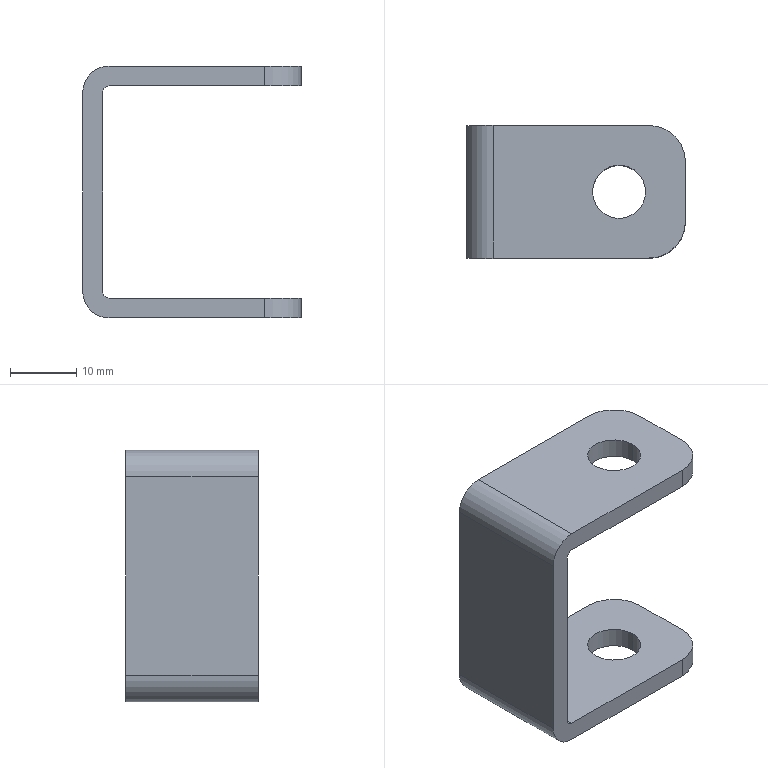Part | NX | features BLEND 1, DATUM_CSYS 1, EXTRACT_DATUM_PLANE 1, EXTRUDE 1, LINKED_BODY 1, SKETCH 1, SUBTRACT 1 | 1 solid | 22 faces | box 33 x 20 x 38 mm | volume 5372 mm3 | cylinder 12 | plane 10 | commonest cylinder face diameters 8 x6 11 x4 2 x2
STEP:
#1=CARTESIAN_POINT('',(-23.,10.,-15.));
#2=VERTEX_POINT('',#1);
#3=CARTESIAN_POINT('',(-23.,10.,15.));
#4=VERTEX_POINT('',#3);
#5=CARTESIAN_POINT('',(-23.,10.,-15.));
#6=DIRECTION('',(0.,0.,1.));
#7=VECTOR('',#6,1000.);
#8=LINE('',#5,#7);
#9=EDGE_CURVE('',#2,#4,#8,.T.);
#10=ORIENTED_EDGE('',*,*,#9,.F.);
#11=CARTESIAN_POINT('',(-23.,-10.,-15.));
#12=VERTEX_POINT('',#11);
#13=CARTESIAN_POINT('',(-23.,-10.,-15.));
#14=DIRECTION('',(0.,1.,0.));
#15=VECTOR('',#14,1000.);
#16=LINE('',#13,#15);
#17=EDGE_CURVE('',#12,#2,#16,.T.);
#18=ORIENTED_EDGE('',*,*,#17,.F.);
#19=CARTESIAN_POINT('',(-23.,-10.,15.));
#20=VERTEX_POINT('',#19);
#21=CARTESIAN_POINT('',(-23.,-10.,-15.));
#22=DIRECTION('',(0.,0.,1.));
#23=VECTOR('',#22,1000.);
#24=LINE('',#21,#23);
#25=EDGE_CURVE('',#12,#20,#24,.T.);
#26=ORIENTED_EDGE('',*,*,#25,.T.);
#27=CARTESIAN_POINT('',(-23.,-10.,15.));
#28=DIRECTION('',(0.,1.,0.));
#29=VECTOR('',#28,1000.);
#30=LINE('',#27,#29);
#31=EDGE_CURVE('',#20,#4,#30,.T.);
#32=ORIENTED_EDGE('',*,*,#31,.T.);
#33=EDGE_LOOP('',(#10,#18,#26,#32));
#34=FACE_BOUND('',#33,.T.);
#35=CARTESIAN_POINT('',(-23.,-10.,-15.));
#36=DIRECTION('',(-1.,0.,0.));
#37=DIRECTION('',(0.,0.,1.));
#38=AXIS2_PLACEMENT_3D('',#35,#36,#37);
#39=PLANE('',#38);
#40=ADVANCED_FACE('',(#34),#39,.T.);
#41=CARTESIAN_POINT('',(-19.,10.,19.));
#42=VERTEX_POINT('',#41);
#43=CARTESIAN_POINT('',(-19.,10.,15.));
#44=DIRECTION('',(0.,1.,0.));
#45=DIRECTION('',(-1.,0.,0.));
#46=AXIS2_PLACEMENT_3D('',#43,#44,#45);
#47=CIRCLE('',#46,4.);
#48=EDGE_CURVE('',#4,#42,#47,.T.);
#49=ORIENTED_EDGE('',*,*,#48,.F.);
#50=ORIENTED_EDGE('',*,*,#31,.F.);
#51=CARTESIAN_POINT('',(-19.,-10.,19.));
#52=VERTEX_POINT('',#51);
#53=CARTESIAN_POINT('',(-19.,-10.,15.));
#54=DIRECTION('',(0.,1.,0.));
#55=DIRECTION('',(-1.,0.,0.));
#56=AXIS2_PLACEMENT_3D('',#53,#54,#55);
#57=CIRCLE('',#56,4.);
#58=EDGE_CURVE('',#20,#52,#57,.T.);
#59=ORIENTED_EDGE('',*,*,#58,.T.);
#60=CARTESIAN_POINT('',(-19.,-10.,19.));
#61=DIRECTION('',(0.,1.,0.));
#62=VECTOR('',#61,1000.);
#63=LINE('',#60,#62);
#64=EDGE_CURVE('',#52,#42,#63,.T.);
#65=ORIENTED_EDGE('',*,*,#64,.T.);
#66=EDGE_LOOP('',(#49,#50,#59,#65));
#67=FACE_BOUND('',#66,.T.);
#68=CARTESIAN_POINT('',(-19.,-10.,15.));
#69=DIRECTION('',(0.,1.,0.));
#70=DIRECTION('',(0.,0.,1.));
#71=AXIS2_PLACEMENT_3D('',#68,#69,#70);
#72=CYLINDRICAL_SURFACE('',#71,4.);
#73=ADVANCED_FACE('',(#67),#72,.T.);
#74=CARTESIAN_POINT('',(4.5,-10.,19.));
#75=VERTEX_POINT('',#74);
#76=CARTESIAN_POINT('',(-19.,-10.,19.));
#77=DIRECTION('',(1.,0.,0.));
#78=VECTOR('',#77,1000.);
#79=LINE('',#76,#78);
#80=EDGE_CURVE('',#52,#75,#79,.T.);
#81=ORIENTED_EDGE('',*,*,#80,.T.);
#82=CARTESIAN_POINT('',(10.,-4.5,19.));
#83=VERTEX_POINT('',#82);
#84=CARTESIAN_POINT('',(4.5,-4.5,19.));
#85=DIRECTION('',(0.,0.,1.));
#86=DIRECTION('',(1.,0.,0.));
#87=AXIS2_PLACEMENT_3D('',#84,#85,#86);
#88=CIRCLE('',#87,5.5);
#89=EDGE_CURVE('',#75,#83,#88,.T.);
#90=ORIENTED_EDGE('',*,*,#89,.T.);
#91=CARTESIAN_POINT('',(10.,4.5,19.));
#92=VERTEX_POINT('',#91);
#93=CARTESIAN_POINT('',(10.,-10.,19.));
#94=DIRECTION('',(0.,1.,0.));
#95=VECTOR('',#94,1000.);
#96=LINE('',#93,#95);
#97=EDGE_CURVE('',#83,#92,#96,.T.);
#98=ORIENTED_EDGE('',*,*,#97,.T.);
#99=CARTESIAN_POINT('',(4.5,10.,19.));
#100=VERTEX_POINT('',#99);
#101=CARTESIAN_POINT('',(4.5,4.5,19.));
#102=DIRECTION('',(0.,0.,1.));
#103=DIRECTION('',(1.,0.,0.));
#104=AXIS2_PLACEMENT_3D('',#101,#102,#103);
#105=CIRCLE('',#104,5.5);
#106=EDGE_CURVE('',#92,#100,#105,.T.);
#107=ORIENTED_EDGE('',*,*,#106,.T.);
#108=CARTESIAN_POINT('',(5.,10.,19.));
#109=DIRECTION('',(1.,0.,0.));
#110=VECTOR('',#109,1000.);
#111=LINE('',#108,#110);
#112=EDGE_CURVE('',#42,#100,#111,.T.);
#113=ORIENTED_EDGE('',*,*,#112,.F.);
#114=ORIENTED_EDGE('',*,*,#64,.F.);
#115=EDGE_LOOP('',(#81,#90,#98,#107,#113,#114));
#116=FACE_BOUND('',#115,.T.);
#117=CARTESIAN_POINT('',(4.,0.,19.));
#118=VERTEX_POINT('',#117);
#119=CARTESIAN_POINT('',(-4.,0.,19.));
#120=VERTEX_POINT('',#119);
#121=CARTESIAN_POINT('',(0.,0.,19.));
#122=DIRECTION('',(0.,0.,1.));
#123=DIRECTION('',(1.,0.,0.));
#124=AXIS2_PLACEMENT_3D('',#121,#122,#123);
#125=CIRCLE('',#124,4.);
#126=EDGE_CURVE('',#118,#120,#125,.T.);
#127=ORIENTED_EDGE('',*,*,#126,.F.);
#128=CARTESIAN_POINT('',(0.,0.,19.));
#129=DIRECTION('',(0.,0.,1.));
#130=DIRECTION('',(-1.,0.,0.));
#131=AXIS2_PLACEMENT_3D('',#128,#129,#130);
#132=CIRCLE('',#131,4.);
#133=EDGE_CURVE('',#120,#118,#132,.T.);
#134=ORIENTED_EDGE('',*,*,#133,.F.);
#135=EDGE_LOOP('',(#127,#134));
#136=FACE_BOUND('',#135,.T.);
#137=CARTESIAN_POINT('',(5.,-10.,19.));
#138=DIRECTION('',(0.,0.,1.));
#139=DIRECTION('',(1.,0.,0.));
#140=AXIS2_PLACEMENT_3D('',#137,#138,#139);
#141=PLANE('',#140);
#142=ADVANCED_FACE('',(#116,#136),#141,.T.);
#143=ORIENTED_EDGE('',*,*,#97,.F.);
#144=CARTESIAN_POINT('',(10.,-4.5,16.));
#145=VERTEX_POINT('',#144);
#146=CARTESIAN_POINT('',(10.,-4.5,16.));
#147=DIRECTION('',(0.,0.,-1.));
#148=VECTOR('',#147,1000.);
#149=LINE('',#146,#148);
#150=EDGE_CURVE('',#83,#145,#149,.T.);
#151=ORIENTED_EDGE('',*,*,#150,.T.);
#152=CARTESIAN_POINT('',(10.,4.5,16.));
#153=VERTEX_POINT('',#152);
#154=CARTESIAN_POINT('',(10.,-10.,16.));
#155=DIRECTION('',(0.,1.,0.));
#156=VECTOR('',#155,1000.);
#157=LINE('',#154,#156);
#158=EDGE_CURVE('',#145,#153,#157,.T.);
#159=ORIENTED_EDGE('',*,*,#158,.T.);
#160=CARTESIAN_POINT('',(10.,4.5,19.));
#161=DIRECTION('',(0.,0.,-1.));
#162=VECTOR('',#161,1000.);
#163=LINE('',#160,#162);
#164=EDGE_CURVE('',#153,#92,#163,.F.);
#165=ORIENTED_EDGE('',*,*,#164,.T.);
#166=EDGE_LOOP('',(#143,#151,#159,#165));
#167=FACE_BOUND('',#166,.T.);
#168=CARTESIAN_POINT('',(10.,-10.,19.));
#169=DIRECTION('',(1.,0.,0.));
#170=DIRECTION('',(0.,0.,-1.));
#171=AXIS2_PLACEMENT_3D('',#168,#169,#170);
#172=PLANE('',#171);
#173=ADVANCED_FACE('',(#167),#172,.T.);
#174=CARTESIAN_POINT('',(-4.,0.,16.));
#175=VERTEX_POINT('',#174);
#176=CARTESIAN_POINT('',(4.,0.,16.));
#177=VERTEX_POINT('',#176);
#178=CARTESIAN_POINT('',(0.,0.,16.));
#179=DIRECTION('',(0.,0.,-1.));
#180=DIRECTION('',(-1.,0.,0.));
#181=AXIS2_PLACEMENT_3D('',#178,#179,#180);
#182=CIRCLE('',#181,4.);
#183=EDGE_CURVE('',#175,#177,#182,.T.);
#184=ORIENTED_EDGE('',*,*,#183,.F.);
#185=CARTESIAN_POINT('',(0.,0.,16.));
#186=DIRECTION('',(0.,0.,-1.));
#187=DIRECTION('',(-1.,0.,0.));
#188=AXIS2_PLACEMENT_3D('',#185,#186,#187);
#189=CIRCLE('',#188,4.);
#190=EDGE_CURVE('',#177,#175,#189,.T.);
#191=ORIENTED_EDGE('',*,*,#190,.F.);
#192=EDGE_LOOP('',(#184,#191));
#193=FACE_BOUND('',#192,.T.);
#194=ORIENTED_EDGE('',*,*,#158,.F.);
#195=CARTESIAN_POINT('',(4.5,-10.,16.));
#196=VERTEX_POINT('',#195);
#197=CARTESIAN_POINT('',(4.5,-4.5,16.));
#198=DIRECTION('',(0.,0.,-1.));
#199=DIRECTION('',(-1.,0.,0.));
#200=AXIS2_PLACEMENT_3D('',#197,#198,#199);
#201=CIRCLE('',#200,5.5);
#202=EDGE_CURVE('',#145,#196,#201,.T.);
#203=ORIENTED_EDGE('',*,*,#202,.T.);
#204=CARTESIAN_POINT('',(-19.,-10.,16.));
#205=VERTEX_POINT('',#204);
#206=CARTESIAN_POINT('',(10.,-10.,16.));
#207=DIRECTION('',(-1.,0.,0.));
#208=VECTOR('',#207,1000.);
#209=LINE('',#206,#208);
#210=EDGE_CURVE('',#196,#205,#209,.T.);
#211=ORIENTED_EDGE('',*,*,#210,.T.);
#212=CARTESIAN_POINT('',(-19.,10.,16.));
#213=VERTEX_POINT('',#212);
#214=CARTESIAN_POINT('',(-19.,-10.,16.));
#215=DIRECTION('',(0.,1.,0.));
#216=VECTOR('',#215,1000.);
#217=LINE('',#214,#216);
#218=EDGE_CURVE('',#205,#213,#217,.T.);
#219=ORIENTED_EDGE('',*,*,#218,.T.);
#220=CARTESIAN_POINT('',(4.5,10.,16.));
#221=VERTEX_POINT('',#220);
#222=CARTESIAN_POINT('',(5.,10.,16.));
#223=DIRECTION('',(-1.,0.,0.));
#224=VECTOR('',#223,1000.);
#225=LINE('',#222,#224);
#226=EDGE_CURVE('',#221,#213,#225,.T.);
#227=ORIENTED_EDGE('',*,*,#226,.F.);
#228=CARTESIAN_POINT('',(4.5,4.5,16.));
#229=DIRECTION('',(0.,0.,-1.));
#230=DIRECTION('',(-1.,0.,0.));
#231=AXIS2_PLACEMENT_3D('',#228,#229,#230);
#232=CIRCLE('',#231,5.5);
#233=EDGE_CURVE('',#221,#153,#232,.T.);
#234=ORIENTED_EDGE('',*,*,#233,.T.);
#235=EDGE_LOOP('',(#194,#203,#211,#219,#227,#234));
#236=FACE_BOUND('',#235,.T.);
#237=CARTESIAN_POINT('',(5.,-10.,16.));
#238=DIRECTION('',(0.,0.,-1.));
#239=DIRECTION('',(-1.,0.,0.));
#240=AXIS2_PLACEMENT_3D('',#237,#238,#239);
#241=PLANE('',#240);
#242=ADVANCED_FACE('',(#193,#236),#241,.T.);
#243=CARTESIAN_POINT('',(-20.,10.,15.));
#244=VERTEX_POINT('',#243);
#245=CARTESIAN_POINT('',(-19.,10.,15.));
#246=DIRECTION('',(0.,-1.,0.));
#247=DIRECTION('',(0.,0.,1.));
#248=AXIS2_PLACEMENT_3D('',#245,#246,#247);
#249=CIRCLE('',#248,1.);
#250=EDGE_CURVE('',#213,#244,#249,.T.);
#251=ORIENTED_EDGE('',*,*,#250,.F.);
#252=ORIENTED_EDGE('',*,*,#218,.F.);
#253=CARTESIAN_POINT('',(-20.,-10.,15.));
#254=VERTEX_POINT('',#253);
#255=CARTESIAN_POINT('',(-19.,-10.,15.));
#256=DIRECTION('',(0.,-1.,0.));
#257=DIRECTION('',(0.,0.,1.));
#258=AXIS2_PLACEMENT_3D('',#255,#256,#257);
#259=CIRCLE('',#258,1.);
#260=EDGE_CURVE('',#205,#254,#259,.T.);
#261=ORIENTED_EDGE('',*,*,#260,.T.);
#262=CARTESIAN_POINT('',(-20.,-10.,15.));
#263=DIRECTION('',(0.,1.,0.));
#264=VECTOR('',#263,1000.);
#265=LINE('',#262,#264);
#266=EDGE_CURVE('',#254,#244,#265,.T.);
#267=ORIENTED_EDGE('',*,*,#266,.T.);
#268=EDGE_LOOP('',(#251,#252,#261,#267));
#269=FACE_BOUND('',#268,.T.);
#270=CARTESIAN_POINT('',(-19.,-10.,15.));
#271=DIRECTION('',(0.,1.,0.));
#272=DIRECTION('',(0.,0.,1.));
#273=AXIS2_PLACEMENT_3D('',#270,#271,#272);
#274=CYLINDRICAL_SURFACE('',#273,1.);
#275=ADVANCED_FACE('',(#269),#274,.F.);
#276=CARTESIAN_POINT('',(-20.,10.,-15.));
#277=VERTEX_POINT('',#276);
#278=CARTESIAN_POINT('',(-20.,10.,15.));
#279=DIRECTION('',(0.,0.,-1.));
#280=VECTOR('',#279,1000.);
#281=LINE('',#278,#280);
#282=EDGE_CURVE('',#244,#277,#281,.T.);
#283=ORIENTED_EDGE('',*,*,#282,.F.);
#284=ORIENTED_EDGE('',*,*,#266,.F.);
#285=CARTESIAN_POINT('',(-20.,-10.,-15.));
#286=VERTEX_POINT('',#285);
#287=CARTESIAN_POINT('',(-20.,-10.,15.));
#288=DIRECTION('',(0.,0.,-1.));
#289=VECTOR('',#288,1000.);
#290=LINE('',#287,#289);
#291=EDGE_CURVE('',#254,#286,#290,.T.);
#292=ORIENTED_EDGE('',*,*,#291,.T.);
#293=CARTESIAN_POINT('',(-20.,-10.,-15.));
#294=DIRECTION('',(0.,1.,0.));
#295=VECTOR('',#294,1000.);
#296=LINE('',#293,#295);
#297=EDGE_CURVE('',#286,#277,#296,.T.);
#298=ORIENTED_EDGE('',*,*,#297,.T.);
#299=EDGE_LOOP('',(#283,#284,#292,#298));
#300=FACE_BOUND('',#299,.T.);
#301=CARTESIAN_POINT('',(-20.,-10.,15.));
#302=DIRECTION('',(1.,0.,0.));
#303=DIRECTION('',(0.,0.,-1.));
#304=AXIS2_PLACEMENT_3D('',#301,#302,#303);
#305=PLANE('',#304);
#306=ADVANCED_FACE('',(#300),#305,.T.);
#307=CARTESIAN_POINT('',(-19.,10.,-16.));
#308=VERTEX_POINT('',#307);
#309=CARTESIAN_POINT('',(-19.,10.,-15.));
#310=DIRECTION('',(0.,-1.,0.));
#311=DIRECTION('',(-1.,0.,0.));
#312=AXIS2_PLACEMENT_3D('',#309,#310,#311);
#313=CIRCLE('',#312,1.);
#314=EDGE_CURVE('',#277,#308,#313,.T.);
#315=ORIENTED_EDGE('',*,*,#314,.F.);
#316=ORIENTED_EDGE('',*,*,#297,.F.);
#317=CARTESIAN_POINT('',(-19.,-10.,-16.));
#318=VERTEX_POINT('',#317);
#319=CARTESIAN_POINT('',(-19.,-10.,-15.));
#320=DIRECTION('',(0.,-1.,0.));
#321=DIRECTION('',(-1.,0.,0.));
#322=AXIS2_PLACEMENT_3D('',#319,#320,#321);
#323=CIRCLE('',#322,1.);
#324=EDGE_CURVE('',#286,#318,#323,.T.);
#325=ORIENTED_EDGE('',*,*,#324,.T.);
#326=CARTESIAN_POINT('',(-19.,-10.,-16.));
#327=DIRECTION('',(0.,1.,0.));
#328=VECTOR('',#327,1000.);
#329=LINE('',#326,#328);
#330=EDGE_CURVE('',#318,#308,#329,.T.);
#331=ORIENTED_EDGE('',*,*,#330,.T.);
#332=EDGE_LOOP('',(#315,#316,#325,#331));
#333=FACE_BOUND('',#332,.T.);
#334=CARTESIAN_POINT('',(-19.,-10.,-15.));
#335=DIRECTION('',(0.,1.,0.));
#336=DIRECTION('',(0.,0.,1.));
#337=AXIS2_PLACEMENT_3D('',#334,#335,#336);
#338=CYLINDRICAL_SURFACE('',#337,1.);
#339=ADVANCED_FACE('',(#333),#338,.F.);
#340=CARTESIAN_POINT('',(4.,0.,-16.));
#341=VERTEX_POINT('',#340);
#342=CARTESIAN_POINT('',(-4.,0.,-16.));
#343=VERTEX_POINT('',#342);
#344=CARTESIAN_POINT('',(0.,0.,-16.));
#345=DIRECTION('',(0.,0.,1.));
#346=DIRECTION('',(1.,0.,0.));
#347=AXIS2_PLACEMENT_3D('',#344,#345,#346);
#348=CIRCLE('',#347,4.);
#349=EDGE_CURVE('',#341,#343,#348,.T.);
#350=ORIENTED_EDGE('',*,*,#349,.F.);
#351=CARTESIAN_POINT('',(0.,0.,-16.));
#352=DIRECTION('',(0.,0.,1.));
#353=DIRECTION('',(1.,0.,0.));
#354=AXIS2_PLACEMENT_3D('',#351,#352,#353);
#355=CIRCLE('',#354,4.);
#356=EDGE_CURVE('',#343,#341,#355,.T.);
#357=ORIENTED_EDGE('',*,*,#356,.F.);
#358=EDGE_LOOP('',(#350,#357));
#359=FACE_BOUND('',#358,.T.);
#360=CARTESIAN_POINT('',(4.5,-10.,-16.));
#361=VERTEX_POINT('',#360);
#362=CARTESIAN_POINT('',(-19.,-10.,-16.));
#363=DIRECTION('',(1.,0.,0.));
#364=VECTOR('',#363,1000.);
#365=LINE('',#362,#364);
#366=EDGE_CURVE('',#318,#361,#365,.T.);
#367=ORIENTED_EDGE('',*,*,#366,.T.);
#368=CARTESIAN_POINT('',(10.,-4.5,-16.));
#369=VERTEX_POINT('',#368);
#370=CARTESIAN_POINT('',(4.5,-4.5,-16.));
#371=DIRECTION('',(0.,0.,1.));
#372=DIRECTION('',(1.,0.,0.));
#373=AXIS2_PLACEMENT_3D('',#370,#371,#372);
#374=CIRCLE('',#373,5.5);
#375=EDGE_CURVE('',#361,#369,#374,.T.);
#376=ORIENTED_EDGE('',*,*,#375,.T.);
#377=CARTESIAN_POINT('',(10.,4.5,-16.));
#378=VERTEX_POINT('',#377);
#379=CARTESIAN_POINT('',(10.,-10.,-16.));
#380=DIRECTION('',(0.,1.,0.));
#381=VECTOR('',#380,1000.);
#382=LINE('',#379,#381);
#383=EDGE_CURVE('',#369,#378,#382,.T.);
#384=ORIENTED_EDGE('',*,*,#383,.T.);
#385=CARTESIAN_POINT('',(4.5,10.,-16.));
#386=VERTEX_POINT('',#385);
#387=CARTESIAN_POINT('',(4.5,4.5,-16.));
#388=DIRECTION('',(0.,0.,1.));
#389=DIRECTION('',(1.,0.,0.));
#390=AXIS2_PLACEMENT_3D('',#387,#388,#389);
#391=CIRCLE('',#390,5.5);
#392=EDGE_CURVE('',#378,#386,#391,.T.);
#393=ORIENTED_EDGE('',*,*,#392,.T.);
#394=CARTESIAN_POINT('',(5.,10.,-16.));
#395=DIRECTION('',(1.,0.,0.));
#396=VECTOR('',#395,1000.);
#397=LINE('',#394,#396);
#398=EDGE_CURVE('',#308,#386,#397,.T.);
#399=ORIENTED_EDGE('',*,*,#398,.F.);
#400=ORIENTED_EDGE('',*,*,#330,.F.);
#401=EDGE_LOOP('',(#367,#376,#384,#393,#399,#400));
#402=FACE_BOUND('',#401,.T.);
#403=CARTESIAN_POINT('',(5.,-10.,-16.));
#404=DIRECTION('',(0.,0.,1.));
#405=DIRECTION('',(1.,0.,0.));
#406=AXIS2_PLACEMENT_3D('',#403,#404,#405);
#407=PLANE('',#406);
#408=ADVANCED_FACE('',(#359,#402),#407,.T.);
#409=ORIENTED_EDGE('',*,*,#383,.F.);
#410=CARTESIAN_POINT('',(10.,-4.5,-19.));
#411=VERTEX_POINT('',#410);
#412=CARTESIAN_POINT('',(10.,-4.5,-19.));
#413=DIRECTION('',(0.,0.,-1.));
#414=VECTOR('',#413,1000.);
#415=LINE('',#412,#414);
#416=EDGE_CURVE('',#369,#411,#415,.T.);
#417=ORIENTED_EDGE('',*,*,#416,.T.);
#418=CARTESIAN_POINT('',(10.,4.5,-19.));
#419=VERTEX_POINT('',#418);
#420=CARTESIAN_POINT('',(10.,-10.,-19.));
#421=DIRECTION('',(0.,1.,0.));
#422=VECTOR('',#421,1000.);
#423=LINE('',#420,#422);
#424=EDGE_CURVE('',#411,#419,#423,.T.);
#425=ORIENTED_EDGE('',*,*,#424,.T.);
#426=CARTESIAN_POINT('',(10.,4.5,-16.));
#427=DIRECTION('',(0.,0.,-1.));
#428=VECTOR('',#427,1000.);
#429=LINE('',#426,#428);
#430=EDGE_CURVE('',#419,#378,#429,.F.);
#431=ORIENTED_EDGE('',*,*,#430,.T.);
#432=EDGE_LOOP('',(#409,#417,#425,#431));
#433=FACE_BOUND('',#432,.T.);
#434=CARTESIAN_POINT('',(10.,-10.,-16.));
#435=DIRECTION('',(1.,0.,0.));
#436=DIRECTION('',(0.,0.,-1.));
#437=AXIS2_PLACEMENT_3D('',#434,#435,#436);
#438=PLANE('',#437);
#439=ADVANCED_FACE('',(#433),#438,.T.);
#440=CARTESIAN_POINT('',(-4.,0.,-19.));
#441=VERTEX_POINT('',#440);
#442=CARTESIAN_POINT('',(4.,0.,-19.));
#443=VERTEX_POINT('',#442);
#444=CARTESIAN_POINT('',(0.,0.,-19.));
#445=DIRECTION('',(0.,0.,-1.));
#446=DIRECTION('',(-1.,0.,0.));
#447=AXIS2_PLACEMENT_3D('',#444,#445,#446);
#448=CIRCLE('',#447,4.);
#449=EDGE_CURVE('',#441,#443,#448,.T.);
#450=ORIENTED_EDGE('',*,*,#449,.F.);
#451=CARTESIAN_POINT('',(0.,0.,-19.));
#452=DIRECTION('',(0.,0.,-1.));
#453=DIRECTION('',(-1.,0.,0.));
#454=AXIS2_PLACEMENT_3D('',#451,#452,#453);
#455=CIRCLE('',#454,4.);
#456=EDGE_CURVE('',#443,#441,#455,.T.);
#457=ORIENTED_EDGE('',*,*,#456,.F.);
#458=EDGE_LOOP('',(#450,#457));
#459=FACE_BOUND('',#458,.T.);
#460=ORIENTED_EDGE('',*,*,#424,.F.);
#461=CARTESIAN_POINT('',(4.5,-10.,-19.));
#462=VERTEX_POINT('',#461);
#463=CARTESIAN_POINT('',(4.5,-4.5,-19.));
#464=DIRECTION('',(0.,0.,-1.));
#465=DIRECTION('',(-1.,0.,0.));
#466=AXIS2_PLACEMENT_3D('',#463,#464,#465);
#467=CIRCLE('',#466,5.5);
#468=EDGE_CURVE('',#411,#462,#467,.T.);
#469=ORIENTED_EDGE('',*,*,#468,.T.);
#470=CARTESIAN_POINT('',(-19.,-10.,-19.));
#471=VERTEX_POINT('',#470);
#472=CARTESIAN_POINT('',(10.,-10.,-19.));
#473=DIRECTION('',(-1.,0.,0.));
#474=VECTOR('',#473,1000.);
#475=LINE('',#472,#474);
#476=EDGE_CURVE('',#462,#471,#475,.T.);
#477=ORIENTED_EDGE('',*,*,#476,.T.);
#478=CARTESIAN_POINT('',(-19.,10.,-19.));
#479=VERTEX_POINT('',#478);
#480=CARTESIAN_POINT('',(-19.,-10.,-19.));
#481=DIRECTION('',(0.,1.,0.));
#482=VECTOR('',#481,1000.);
#483=LINE('',#480,#482);
#484=EDGE_CURVE('',#471,#479,#483,.T.);
#485=ORIENTED_EDGE('',*,*,#484,.T.);
#486=CARTESIAN_POINT('',(4.5,10.,-19.));
#487=VERTEX_POINT('',#486);
#488=CARTESIAN_POINT('',(5.,10.,-19.));
#489=DIRECTION('',(-1.,0.,0.));
#490=VECTOR('',#489,1000.);
#491=LINE('',#488,#490);
#492=EDGE_CURVE('',#487,#479,#491,.T.);
#493=ORIENTED_EDGE('',*,*,#492,.F.);
#494=CARTESIAN_POINT('',(4.5,4.5,-19.));
#495=DIRECTION('',(0.,0.,-1.));
#496=DIRECTION('',(-1.,0.,0.));
#497=AXIS2_PLACEMENT_3D('',#494,#495,#496);
#498=CIRCLE('',#497,5.5);
#499=EDGE_CURVE('',#487,#419,#498,.T.);
#500=ORIENTED_EDGE('',*,*,#499,.T.);
#501=EDGE_LOOP('',(#460,#469,#477,#485,#493,#500));
#502=FACE_BOUND('',#501,.T.);
#503=CARTESIAN_POINT('',(5.,-10.,-19.));
#504=DIRECTION('',(0.,0.,-1.));
#505=DIRECTION('',(-1.,0.,0.));
#506=AXIS2_PLACEMENT_3D('',#503,#504,#505);
#507=PLANE('',#506);
#508=ADVANCED_FACE('',(#459,#502),#507,.T.);
#509=CARTESIAN_POINT('',(-19.,10.,-15.));
#510=DIRECTION('',(0.,1.,0.));
#511=DIRECTION('',(0.,0.,-1.));
#512=AXIS2_PLACEMENT_3D('',#509,#510,#511);
#513=CIRCLE('',#512,4.);
#514=EDGE_CURVE('',#479,#2,#513,.T.);
#515=ORIENTED_EDGE('',*,*,#514,.F.);
#516=ORIENTED_EDGE('',*,*,#484,.F.);
#517=CARTESIAN_POINT('',(-19.,-10.,-15.));
#518=DIRECTION('',(0.,1.,0.));
#519=DIRECTION('',(0.,0.,-1.));
#520=AXIS2_PLACEMENT_3D('',#517,#518,#519);
#521=CIRCLE('',#520,4.);
#522=EDGE_CURVE('',#471,#12,#521,.T.);
#523=ORIENTED_EDGE('',*,*,#522,.T.);
#524=ORIENTED_EDGE('',*,*,#17,.T.);
#525=EDGE_LOOP('',(#515,#516,#523,#524));
#526=FACE_BOUND('',#525,.T.);
#527=CARTESIAN_POINT('',(-19.,-10.,-15.));
#528=DIRECTION('',(0.,1.,0.));
#529=DIRECTION('',(0.,0.,1.));
#530=AXIS2_PLACEMENT_3D('',#527,#528,#529);
#531=CYLINDRICAL_SURFACE('',#530,4.);
#532=ADVANCED_FACE('',(#526),#531,.T.);
#533=ORIENTED_EDGE('',*,*,#476,.F.);
#534=CARTESIAN_POINT('',(4.5,-10.,-16.));
#535=DIRECTION('',(0.,0.,-1.));
#536=VECTOR('',#535,1000.);
#537=LINE('',#534,#536);
#538=EDGE_CURVE('',#462,#361,#537,.F.);
#539=ORIENTED_EDGE('',*,*,#538,.T.);
#540=ORIENTED_EDGE('',*,*,#366,.F.);
#541=ORIENTED_EDGE('',*,*,#324,.F.);
#542=ORIENTED_EDGE('',*,*,#291,.F.);
#543=ORIENTED_EDGE('',*,*,#260,.F.);
#544=ORIENTED_EDGE('',*,*,#210,.F.);
#545=CARTESIAN_POINT('',(4.5,-10.,19.));
#546=DIRECTION('',(0.,0.,-1.));
#547=VECTOR('',#546,1000.);
#548=LINE('',#545,#547);
#549=EDGE_CURVE('',#196,#75,#548,.F.);
#550=ORIENTED_EDGE('',*,*,#549,.T.);
#551=ORIENTED_EDGE('',*,*,#80,.F.);
#552=ORIENTED_EDGE('',*,*,#58,.F.);
#553=ORIENTED_EDGE('',*,*,#25,.F.);
#554=ORIENTED_EDGE('',*,*,#522,.F.);
#555=EDGE_LOOP('',(#533,#539,#540,#541,#542,#543,#544,#550,#551,#552,#553,#554));
#556=FACE_BOUND('',#555,.T.);
#557=CARTESIAN_POINT('',(-19.,-10.,15.));
#558=DIRECTION('',(0.,1.,0.));
#559=DIRECTION('',(0.,0.,1.));
#560=AXIS2_PLACEMENT_3D('',#557,#558,#559);
#561=PLANE('',#560);
#562=ADVANCED_FACE('',(#556),#561,.F.);
#563=ORIENTED_EDGE('',*,*,#398,.T.);
#564=CARTESIAN_POINT('',(4.5,10.,15.));
#565=DIRECTION('',(0.,0.,-1.));
#566=VECTOR('',#565,1000.);
#567=LINE('',#564,#566);
#568=EDGE_CURVE('',#386,#487,#567,.T.);
#569=ORIENTED_EDGE('',*,*,#568,.T.);
#570=ORIENTED_EDGE('',*,*,#492,.T.);
#571=ORIENTED_EDGE('',*,*,#514,.T.);
#572=ORIENTED_EDGE('',*,*,#9,.T.);
#573=ORIENTED_EDGE('',*,*,#48,.T.);
#574=ORIENTED_EDGE('',*,*,#112,.T.);
#575=CARTESIAN_POINT('',(4.5,10.,15.));
#576=DIRECTION('',(0.,0.,-1.));
#577=VECTOR('',#576,1000.);
#578=LINE('',#575,#577);
#579=EDGE_CURVE('',#100,#221,#578,.T.);
#580=ORIENTED_EDGE('',*,*,#579,.T.);
#581=ORIENTED_EDGE('',*,*,#226,.T.);
#582=ORIENTED_EDGE('',*,*,#250,.T.);
#583=ORIENTED_EDGE('',*,*,#282,.T.);
#584=ORIENTED_EDGE('',*,*,#314,.T.);
#585=EDGE_LOOP('',(#563,#569,#570,#571,#572,#573,#574,#580,#581,#582,#583,#584));
#586=FACE_BOUND('',#585,.T.);
#587=CARTESIAN_POINT('',(-19.,10.,15.));
#588=DIRECTION('',(0.,1.,0.));
#589=DIRECTION('',(0.,0.,1.));
#590=AXIS2_PLACEMENT_3D('',#587,#588,#589);
#591=PLANE('',#590);
#592=ADVANCED_FACE('',(#586),#591,.T.);
#593=ORIENTED_EDGE('',*,*,#375,.F.);
#594=ORIENTED_EDGE('',*,*,#538,.F.);
#595=ORIENTED_EDGE('',*,*,#468,.F.);
#596=ORIENTED_EDGE('',*,*,#416,.F.);
#597=EDGE_LOOP('',(#593,#594,#595,#596));
#598=FACE_BOUND('',#597,.T.);
#599=CARTESIAN_POINT('',(4.5,-4.5,-16.));
#600=DIRECTION('',(0.,0.,1.));
#601=DIRECTION('',(1.,0.,0.));
#602=AXIS2_PLACEMENT_3D('',#599,#600,#601);
#603=CYLINDRICAL_SURFACE('',#602,5.5);
#604=ADVANCED_FACE('',(#598),#603,.T.);
#605=ORIENTED_EDGE('',*,*,#392,.F.);
#606=ORIENTED_EDGE('',*,*,#430,.F.);
#607=ORIENTED_EDGE('',*,*,#499,.F.);
#608=ORIENTED_EDGE('',*,*,#568,.F.);
#609=EDGE_LOOP('',(#605,#606,#607,#608));
#610=FACE_BOUND('',#609,.T.);
#611=CARTESIAN_POINT('',(4.5,4.5,15.));
#612=DIRECTION('',(0.,0.,-1.));
#613=DIRECTION('',(-1.,0.,0.));
#614=AXIS2_PLACEMENT_3D('',#611,#612,#613);
#615=CYLINDRICAL_SURFACE('',#614,5.5);
#616=ADVANCED_FACE('',(#610),#615,.T.);
#617=ORIENTED_EDGE('',*,*,#89,.F.);
#618=ORIENTED_EDGE('',*,*,#549,.F.);
#619=ORIENTED_EDGE('',*,*,#202,.F.);
#620=ORIENTED_EDGE('',*,*,#150,.F.);
#621=EDGE_LOOP('',(#617,#618,#619,#620));
#622=FACE_BOUND('',#621,.T.);
#623=CARTESIAN_POINT('',(4.5,-4.5,19.));
#624=DIRECTION('',(0.,0.,1.));
#625=DIRECTION('',(1.,0.,0.));
#626=AXIS2_PLACEMENT_3D('',#623,#624,#625);
#627=CYLINDRICAL_SURFACE('',#626,5.5);
#628=ADVANCED_FACE('',(#622),#627,.T.);
#629=ORIENTED_EDGE('',*,*,#106,.F.);
#630=ORIENTED_EDGE('',*,*,#164,.F.);
#631=ORIENTED_EDGE('',*,*,#233,.F.);
#632=ORIENTED_EDGE('',*,*,#579,.F.);
#633=EDGE_LOOP('',(#629,#630,#631,#632));
#634=FACE_BOUND('',#633,.T.);
#635=CARTESIAN_POINT('',(4.5,4.5,15.));
#636=DIRECTION('',(0.,0.,-1.));
#637=DIRECTION('',(-1.,0.,0.));
#638=AXIS2_PLACEMENT_3D('',#635,#636,#637);
#639=CYLINDRICAL_SURFACE('',#638,5.5);
#640=ADVANCED_FACE('',(#634),#639,.T.);
#641=ORIENTED_EDGE('',*,*,#356,.T.);
#642=CARTESIAN_POINT('',(4.,0.,-25.));
#643=DIRECTION('',(0.,0.,1.));
#644=VECTOR('',#643,1000.);
#645=LINE('',#642,#644);
#646=EDGE_CURVE('',#341,#443,#645,.F.);
#647=ORIENTED_EDGE('',*,*,#646,.T.);
#648=ORIENTED_EDGE('',*,*,#456,.T.);
#649=CARTESIAN_POINT('',(-4.,0.,-25.));
#650=DIRECTION('',(0.,0.,1.));
#651=VECTOR('',#650,1000.);
#652=LINE('',#649,#651);
#653=EDGE_CURVE('',#343,#441,#652,.F.);
#654=ORIENTED_EDGE('',*,*,#653,.F.);
#655=EDGE_LOOP('',(#641,#647,#648,#654));
#656=FACE_BOUND('',#655,.T.);
#657=CARTESIAN_POINT('',(0.,0.,19.));
#658=DIRECTION('',(0.,0.,-1.));
#659=DIRECTION('',(1.,0.,0.));
#660=AXIS2_PLACEMENT_3D('',#657,#658,#659);
#661=CYLINDRICAL_SURFACE('',#660,4.);
#662=ADVANCED_FACE('',(#656),#661,.F.);
#663=ORIENTED_EDGE('',*,*,#349,.T.);
#664=ORIENTED_EDGE('',*,*,#653,.T.);
#665=ORIENTED_EDGE('',*,*,#449,.T.);
#666=ORIENTED_EDGE('',*,*,#646,.F.);
#667=EDGE_LOOP('',(#663,#664,#665,#666));
#668=FACE_BOUND('',#667,.T.);
#669=CARTESIAN_POINT('',(0.,0.,19.));
#670=DIRECTION('',(0.,0.,-1.));
#671=DIRECTION('',(1.,0.,0.));
#672=AXIS2_PLACEMENT_3D('',#669,#670,#671);
#673=CYLINDRICAL_SURFACE('',#672,4.);
#674=ADVANCED_FACE('',(#668),#673,.F.);
#675=ORIENTED_EDGE('',*,*,#183,.T.);
#676=CARTESIAN_POINT('',(4.,0.,-25.));
#677=DIRECTION('',(0.,0.,1.));
#678=VECTOR('',#677,1000.);
#679=LINE('',#676,#678);
#680=EDGE_CURVE('',#177,#118,#679,.T.);
#681=ORIENTED_EDGE('',*,*,#680,.T.);
#682=ORIENTED_EDGE('',*,*,#126,.T.);
#683=CARTESIAN_POINT('',(-4.,0.,-25.));
#684=DIRECTION('',(0.,0.,1.));
#685=VECTOR('',#684,1000.);
#686=LINE('',#683,#685);
#687=EDGE_CURVE('',#120,#175,#686,.F.);
#688=ORIENTED_EDGE('',*,*,#687,.T.);
#689=EDGE_LOOP('',(#675,#681,#682,#688));
#690=FACE_BOUND('',#689,.T.);
#691=CARTESIAN_POINT('',(0.,0.,19.));
#692=DIRECTION('',(0.,0.,-1.));
#693=DIRECTION('',(1.,0.,0.));
#694=AXIS2_PLACEMENT_3D('',#691,#692,#693);
#695=CYLINDRICAL_SURFACE('',#694,4.);
#696=ADVANCED_FACE('',(#690),#695,.F.);
#697=ORIENTED_EDGE('',*,*,#190,.T.);
#698=ORIENTED_EDGE('',*,*,#687,.F.);
#699=ORIENTED_EDGE('',*,*,#133,.T.);
#700=ORIENTED_EDGE('',*,*,#680,.F.);
#701=EDGE_LOOP('',(#697,#698,#699,#700));
#702=FACE_BOUND('',#701,.T.);
#703=CARTESIAN_POINT('',(0.,0.,19.));
#704=DIRECTION('',(0.,0.,-1.));
#705=DIRECTION('',(1.,0.,0.));
#706=AXIS2_PLACEMENT_3D('',#703,#704,#705);
#707=CYLINDRICAL_SURFACE('',#706,4.);
#708=ADVANCED_FACE('',(#702),#707,.F.);
#709=CLOSED_SHELL('',(#40,#73,#142,#173,#242,#275,#306,#339,#408,#439,#508,#532,#562,#592,#604,#616,#628,#640,#662,#674,#696,#708));
#710=MANIFOLD_SOLID_BREP('',#709);
#711=(LENGTH_UNIT()NAMED_UNIT(*)SI_UNIT(.MILLI.,.METRE.));
#712=UNCERTAINTY_MEASURE_WITH_UNIT(LENGTH_MEASURE(0.00001),#711,'','');
#713=(NAMED_UNIT(*)PLANE_ANGLE_UNIT()SI_UNIT($,.RADIAN.));
#714=(NAMED_UNIT(*)SI_UNIT($,.STERADIAN.)SOLID_ANGLE_UNIT());
#715=(GEOMETRIC_REPRESENTATION_CONTEXT(3)GLOBAL_UNCERTAINTY_ASSIGNED_CONTEXT((#712))GLOBAL_UNIT_ASSIGNED_CONTEXT((#711,#713,#714))REPRESENTATION_CONTEXT('',''));
#716=ADVANCED_BREP_SHAPE_REPRESENTATION('',(#710),#715);